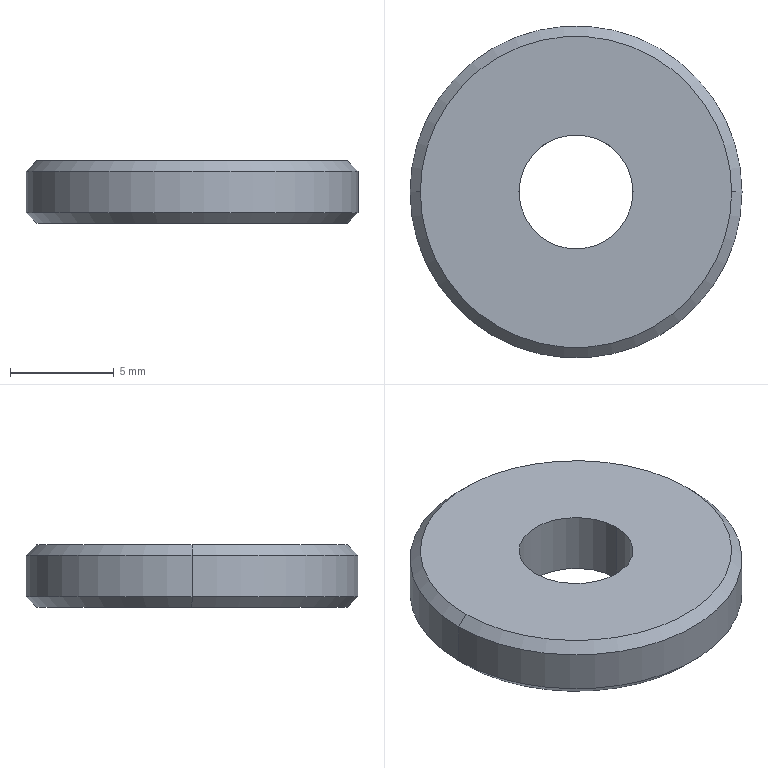Part | STEP file | 1 solid | 10 faces | box 16 x 16 x 3 mm | volume 519.606 mm3 | cone 4 | cylinder 4 | plane 2 | commonest cylinder face diameters 5.5 x2 16 x2
STEP:
#1=CARTESIAN_POINT('',(0.,0.,0.));
#2=DIRECTION('',(0.,0.,1.));
#3=DIRECTION('',(1.,0.,0.));
#4=AXIS2_PLACEMENT_3D('',#1,#2,#3);
#5=CARTESIAN_POINT('',(-7.5,0.,0.));
#6=VERTEX_POINT('',#5);
#7=CARTESIAN_POINT('',(7.5,0.,0.));
#8=VERTEX_POINT('',#7);
#9=CARTESIAN_POINT('',(0.,0.,0.));
#10=DIRECTION('',(0.,0.,-1.));
#11=DIRECTION('',(1.,0.,0.));
#12=AXIS2_PLACEMENT_3D('',#9,#10,#11);
#13=CIRCLE('',#12,7.5);
#14=CARTESIAN_POINT('',(0.,0.,0.5));
#15=DIRECTION('',(0.,0.,1.));
#16=DIRECTION('',(1.,0.,0.));
#17=AXIS2_PLACEMENT_3D('',#14,#15,#16);
#18=CONICAL_SURFACE('',#17,8.,0.7854);
#19=CARTESIAN_POINT('',(6.283,-0.5));
#20=DIRECTION('',(-1.,0.));
#21=VECTOR('',#20,1.);
#22=LINE('',#19,#21);
#23=(GEOMETRIC_REPRESENTATION_CONTEXT(2)PARAMETRIC_REPRESENTATION_CONTEXT()REPRESENTATION_CONTEXT('',''));
#24=DEFINITIONAL_REPRESENTATION('',(#22),#23);
#25=PCURVE('',#18,#24);
#26=CARTESIAN_POINT('',(0.,0.,0.));
#27=DIRECTION('',(0.,0.,1.));
#28=DIRECTION('',(1.,0.,0.));
#29=AXIS2_PLACEMENT_3D('',#26,#27,#28);
#30=PLANE('',#29);
#31=CARTESIAN_POINT('',(7.5,0.));
#32=CARTESIAN_POINT('',(7.5,-12.99));
#33=CARTESIAN_POINT('',(-3.75,-6.495));
#34=CARTESIAN_POINT('',(-15.,0.));
#35=CARTESIAN_POINT('',(-3.75,6.495));
#36=CARTESIAN_POINT('',(7.5,12.99));
#37=CARTESIAN_POINT('',(7.5,0.));
#38=(BOUNDED_CURVE()B_SPLINE_CURVE(2,(#31,#32,#33,#34,#35,#36,#37),.UNSPECIFIED.,.T.,.F.)B_SPLINE_CURVE_WITH_KNOTS((1,2,2,2,2,1),(-2.094,0.,2.094,4.189,6.283,8.378),.UNSPECIFIED.)CURVE()GEOMETRIC_REPRESENTATION_ITEM()RATIONAL_B_SPLINE_CURVE((1.,0.5,1.,0.5,1.,0.5,1.))REPRESENTATION_ITEM(''));
#39=(GEOMETRIC_REPRESENTATION_CONTEXT(2)PARAMETRIC_REPRESENTATION_CONTEXT()REPRESENTATION_CONTEXT('',''));
#40=DEFINITIONAL_REPRESENTATION('',(#38),#39);
#41=PCURVE('',#30,#40);
#42=SURFACE_CURVE('',#13,(#25,#41),.PCURVE_S1.);
#43=EDGE_CURVE('',#6,#8,#42,.T.);
#44=ORIENTED_EDGE('',*,*,#43,.F.);
#45=CARTESIAN_POINT('',(-8.,0.,0.5));
#46=VERTEX_POINT('',#45);
#47=CARTESIAN_POINT('',(-8.,0.,0.5));
#48=DIRECTION('',(-0.7071,0.,0.7071));
#49=VECTOR('',#48,1.);
#50=LINE('',#47,#49);
#51=CARTESIAN_POINT('',(3.142,0.));
#52=DIRECTION('',(0.,1.));
#53=VECTOR('',#52,1.);
#54=LINE('',#51,#53);
#55=(GEOMETRIC_REPRESENTATION_CONTEXT(2)PARAMETRIC_REPRESENTATION_CONTEXT()REPRESENTATION_CONTEXT('',''));
#56=DEFINITIONAL_REPRESENTATION('',(#54),#55);
#57=PCURVE('',#18,#56);
#58=CARTESIAN_POINT('',(0.,0.,0.5));
#59=DIRECTION('',(0.,0.,1.));
#60=DIRECTION('',(1.,0.,0.));
#61=AXIS2_PLACEMENT_3D('',#58,#59,#60);
#62=CONICAL_SURFACE('',#61,8.,0.7854);
#63=CARTESIAN_POINT('',(3.142,0.));
#64=DIRECTION('',(0.,1.));
#65=VECTOR('',#64,1.);
#66=LINE('',#63,#65);
#67=(GEOMETRIC_REPRESENTATION_CONTEXT(2)PARAMETRIC_REPRESENTATION_CONTEXT()REPRESENTATION_CONTEXT('',''));
#68=DEFINITIONAL_REPRESENTATION('',(#66),#67);
#69=PCURVE('',#62,#68);
#70=SURFACE_CURVE('',#50,(#57,#69),.PCURVE_S1.);
#71=EDGE_CURVE('',#6,#46,#70,.T.);
#72=ORIENTED_EDGE('',*,*,#71,.T.);
#73=CARTESIAN_POINT('',(8.,0.,0.5));
#74=VERTEX_POINT('',#73);
#75=CARTESIAN_POINT('',(0.,0.,0.5));
#76=DIRECTION('',(0.,0.,1.));
#77=DIRECTION('',(1.,0.,0.));
#78=AXIS2_PLACEMENT_3D('',#75,#76,#77);
#79=CIRCLE('',#78,8.);
#80=CARTESIAN_POINT('',(0.,0.));
#81=DIRECTION('',(1.,0.));
#82=VECTOR('',#81,1.);
#83=LINE('',#80,#82);
#84=(GEOMETRIC_REPRESENTATION_CONTEXT(2)PARAMETRIC_REPRESENTATION_CONTEXT()REPRESENTATION_CONTEXT('',''));
#85=DEFINITIONAL_REPRESENTATION('',(#83),#84);
#86=PCURVE('',#18,#85);
#87=CARTESIAN_POINT('',(0.,0.,3.));
#88=DIRECTION('',(0.,0.,-1.));
#89=DIRECTION('',(-1.,0.,0.));
#90=AXIS2_PLACEMENT_3D('',#87,#88,#89);
#91=CYLINDRICAL_SURFACE('',#90,8.);
#92=CARTESIAN_POINT('',(3.142,2.5));
#93=DIRECTION('',(-1.,0.));
#94=VECTOR('',#93,1.);
#95=LINE('',#92,#94);
#96=(GEOMETRIC_REPRESENTATION_CONTEXT(2)PARAMETRIC_REPRESENTATION_CONTEXT()REPRESENTATION_CONTEXT('',''));
#97=DEFINITIONAL_REPRESENTATION('',(#95),#96);
#98=PCURVE('',#91,#97);
#99=SURFACE_CURVE('',#79,(#86,#98),.PCURVE_S1.);
#100=EDGE_CURVE('',#74,#46,#99,.T.);
#101=ORIENTED_EDGE('',*,*,#100,.F.);
#102=CARTESIAN_POINT('',(8.,0.,0.5));
#103=DIRECTION('',(0.7071,0.,0.7071));
#104=VECTOR('',#103,1.);
#105=LINE('',#102,#104);
#106=CARTESIAN_POINT('',(0.,0.));
#107=DIRECTION('',(0.,1.));
#108=VECTOR('',#107,1.);
#109=LINE('',#106,#108);
#110=(GEOMETRIC_REPRESENTATION_CONTEXT(2)PARAMETRIC_REPRESENTATION_CONTEXT()REPRESENTATION_CONTEXT('',''));
#111=DEFINITIONAL_REPRESENTATION('',(#109),#110);
#112=PCURVE('',#18,#111);
#113=CARTESIAN_POINT('',(6.283,0.));
#114=DIRECTION('',(0.,1.));
#115=VECTOR('',#114,1.);
#116=LINE('',#113,#115);
#117=(GEOMETRIC_REPRESENTATION_CONTEXT(2)PARAMETRIC_REPRESENTATION_CONTEXT()REPRESENTATION_CONTEXT('',''));
#118=DEFINITIONAL_REPRESENTATION('',(#116),#117);
#119=PCURVE('',#62,#118);
#120=SURFACE_CURVE('',#105,(#112,#119),.PCURVE_S1.);
#121=EDGE_CURVE('',#8,#74,#120,.T.);
#122=ORIENTED_EDGE('',*,*,#121,.F.);
#123=EDGE_LOOP('',(#44,#72,#101,#122));
#124=FACE_BOUND('',#123,.T.);
#125=ADVANCED_FACE('',(#124),#18,.T.);
#126=CARTESIAN_POINT('',(7.5,0.,3.));
#127=VERTEX_POINT('',#126);
#128=CARTESIAN_POINT('',(-7.5,0.,3.));
#129=VERTEX_POINT('',#128);
#130=CARTESIAN_POINT('',(0.,0.,3.));
#131=DIRECTION('',(0.,0.,1.));
#132=DIRECTION('',(1.,0.,0.));
#133=AXIS2_PLACEMENT_3D('',#130,#131,#132);
#134=CIRCLE('',#133,7.5);
#135=CARTESIAN_POINT('',(0.,0.,3.));
#136=DIRECTION('',(0.,0.,-1.));
#137=DIRECTION('',(-1.,0.,0.));
#138=AXIS2_PLACEMENT_3D('',#135,#136,#137);
#139=CONICAL_SURFACE('',#138,7.5,0.7854);
#140=CARTESIAN_POINT('',(3.142,0.));
#141=DIRECTION('',(-1.,0.));
#142=VECTOR('',#141,1.);
#143=LINE('',#140,#142);
#144=(GEOMETRIC_REPRESENTATION_CONTEXT(2)PARAMETRIC_REPRESENTATION_CONTEXT()REPRESENTATION_CONTEXT('',''));
#145=DEFINITIONAL_REPRESENTATION('',(#143),#144);
#146=PCURVE('',#139,#145);
#147=CARTESIAN_POINT('',(0.,0.,3.));
#148=DIRECTION('',(0.,0.,1.));
#149=DIRECTION('',(1.,0.,0.));
#150=AXIS2_PLACEMENT_3D('',#147,#148,#149);
#151=PLANE('',#150);
#152=CARTESIAN_POINT('',(0.,0.));
#153=DIRECTION('',(1.,0.));
#154=AXIS2_PLACEMENT_2D('',#152,#153);
#155=CIRCLE('',#154,7.5);
#156=(GEOMETRIC_REPRESENTATION_CONTEXT(2)PARAMETRIC_REPRESENTATION_CONTEXT()REPRESENTATION_CONTEXT('',''));
#157=DEFINITIONAL_REPRESENTATION('',(#155),#156);
#158=PCURVE('',#151,#157);
#159=SURFACE_CURVE('',#134,(#146,#158),.PCURVE_S1.);
#160=EDGE_CURVE('',#127,#129,#159,.T.);
#161=ORIENTED_EDGE('',*,*,#160,.F.);
#162=CARTESIAN_POINT('',(8.,0.,2.5));
#163=VERTEX_POINT('',#162);
#164=CARTESIAN_POINT('',(7.5,0.,3.));
#165=DIRECTION('',(0.7071,0.,-0.7071));
#166=VECTOR('',#165,1.);
#167=LINE('',#164,#166);
#168=CARTESIAN_POINT('',(3.142,0.));
#169=DIRECTION('',(0.,1.));
#170=VECTOR('',#169,1.);
#171=LINE('',#168,#170);
#172=(GEOMETRIC_REPRESENTATION_CONTEXT(2)PARAMETRIC_REPRESENTATION_CONTEXT()REPRESENTATION_CONTEXT('',''));
#173=DEFINITIONAL_REPRESENTATION('',(#171),#172);
#174=PCURVE('',#139,#173);
#175=CARTESIAN_POINT('',(0.,0.,3.));
#176=DIRECTION('',(0.,0.,-1.));
#177=DIRECTION('',(-1.,0.,0.));
#178=AXIS2_PLACEMENT_3D('',#175,#176,#177);
#179=CONICAL_SURFACE('',#178,7.5,0.7854);
#180=CARTESIAN_POINT('',(3.142,0.));
#181=DIRECTION('',(0.,1.));
#182=VECTOR('',#181,1.);
#183=LINE('',#180,#182);
#184=(GEOMETRIC_REPRESENTATION_CONTEXT(2)PARAMETRIC_REPRESENTATION_CONTEXT()REPRESENTATION_CONTEXT('',''));
#185=DEFINITIONAL_REPRESENTATION('',(#183),#184);
#186=PCURVE('',#179,#185);
#187=SURFACE_CURVE('',#167,(#174,#186),.PCURVE_S1.);
#188=EDGE_CURVE('',#127,#163,#187,.T.);
#189=ORIENTED_EDGE('',*,*,#188,.T.);
#190=CARTESIAN_POINT('',(-8.,0.,2.5));
#191=VERTEX_POINT('',#190);
#192=CARTESIAN_POINT('',(0.,0.,2.5));
#193=DIRECTION('',(0.,0.,-1.));
#194=DIRECTION('',(1.,0.,0.));
#195=AXIS2_PLACEMENT_3D('',#192,#193,#194);
#196=CIRCLE('',#195,8.);
#197=CARTESIAN_POINT('',(-3.142,0.5));
#198=DIRECTION('',(1.,0.));
#199=VECTOR('',#198,1.);
#200=LINE('',#197,#199);
#201=(GEOMETRIC_REPRESENTATION_CONTEXT(2)PARAMETRIC_REPRESENTATION_CONTEXT()REPRESENTATION_CONTEXT('',''));
#202=DEFINITIONAL_REPRESENTATION('',(#200),#201);
#203=PCURVE('',#139,#202);
#204=CARTESIAN_POINT('',(-3.142,0.5));
#205=DIRECTION('',(1.,0.));
#206=VECTOR('',#205,1.);
#207=LINE('',#204,#206);
#208=(GEOMETRIC_REPRESENTATION_CONTEXT(2)PARAMETRIC_REPRESENTATION_CONTEXT()REPRESENTATION_CONTEXT('',''));
#209=DEFINITIONAL_REPRESENTATION('',(#207),#208);
#210=PCURVE('',#91,#209);
#211=SURFACE_CURVE('',#196,(#203,#210),.PCURVE_S1.);
#212=EDGE_CURVE('',#191,#163,#211,.T.);
#213=ORIENTED_EDGE('',*,*,#212,.F.);
#214=CARTESIAN_POINT('',(-7.5,0.,3.));
#215=DIRECTION('',(-0.7071,0.,-0.7071));
#216=VECTOR('',#215,1.);
#217=LINE('',#214,#216);
#218=CARTESIAN_POINT('',(0.,0.));
#219=DIRECTION('',(0.,1.));
#220=VECTOR('',#219,1.);
#221=LINE('',#218,#220);
#222=(GEOMETRIC_REPRESENTATION_CONTEXT(2)PARAMETRIC_REPRESENTATION_CONTEXT()REPRESENTATION_CONTEXT('',''));
#223=DEFINITIONAL_REPRESENTATION('',(#221),#222);
#224=PCURVE('',#139,#223);
#225=CARTESIAN_POINT('',(6.283,0.));
#226=DIRECTION('',(0.,1.));
#227=VECTOR('',#226,1.);
#228=LINE('',#225,#227);
#229=(GEOMETRIC_REPRESENTATION_CONTEXT(2)PARAMETRIC_REPRESENTATION_CONTEXT()REPRESENTATION_CONTEXT('',''));
#230=DEFINITIONAL_REPRESENTATION('',(#228),#229);
#231=PCURVE('',#179,#230);
#232=SURFACE_CURVE('',#217,(#224,#231),.PCURVE_S1.);
#233=EDGE_CURVE('',#129,#191,#232,.T.);
#234=ORIENTED_EDGE('',*,*,#233,.F.);
#235=EDGE_LOOP('',(#161,#189,#213,#234));
#236=FACE_BOUND('',#235,.T.);
#237=ADVANCED_FACE('',(#236),#139,.T.);
#238=CARTESIAN_POINT('',(-2.75,0.,3.));
#239=VERTEX_POINT('',#238);
#240=CARTESIAN_POINT('',(-2.75,0.,0.));
#241=VERTEX_POINT('',#240);
#242=CARTESIAN_POINT('',(-2.75,0.,3.));
#243=DIRECTION('',(0.,0.,-1.));
#244=VECTOR('',#243,1.);
#245=LINE('',#242,#244);
#246=CARTESIAN_POINT('',(0.,0.,3.));
#247=DIRECTION('',(0.,0.,-1.));
#248=DIRECTION('',(-1.,0.,0.));
#249=AXIS2_PLACEMENT_3D('',#246,#247,#248);
#250=CYLINDRICAL_SURFACE('',#249,2.75);
#251=CARTESIAN_POINT('',(6.283,0.));
#252=DIRECTION('',(0.,1.));
#253=VECTOR('',#252,1.);
#254=LINE('',#251,#253);
#255=(GEOMETRIC_REPRESENTATION_CONTEXT(2)PARAMETRIC_REPRESENTATION_CONTEXT()REPRESENTATION_CONTEXT('',''));
#256=DEFINITIONAL_REPRESENTATION('',(#254),#255);
#257=PCURVE('',#250,#256);
#258=CARTESIAN_POINT('',(0.,0.,3.));
#259=DIRECTION('',(0.,0.,-1.));
#260=DIRECTION('',(-1.,0.,0.));
#261=AXIS2_PLACEMENT_3D('',#258,#259,#260);
#262=CYLINDRICAL_SURFACE('',#261,2.75);
#263=CARTESIAN_POINT('',(0.,0.));
#264=DIRECTION('',(0.,1.));
#265=VECTOR('',#264,1.);
#266=LINE('',#263,#265);
#267=(GEOMETRIC_REPRESENTATION_CONTEXT(2)PARAMETRIC_REPRESENTATION_CONTEXT()REPRESENTATION_CONTEXT('',''));
#268=DEFINITIONAL_REPRESENTATION('',(#266),#267);
#269=PCURVE('',#262,#268);
#270=SURFACE_CURVE('',#245,(#257,#269),.PCURVE_S1.);
#271=EDGE_CURVE('',#239,#241,#270,.T.);
#272=ORIENTED_EDGE('',*,*,#271,.T.);
#273=CARTESIAN_POINT('',(2.75,0.,0.));
#274=VERTEX_POINT('',#273);
#275=CARTESIAN_POINT('',(0.,0.,0.));
#276=DIRECTION('',(0.,0.,1.));
#277=DIRECTION('',(1.,0.,0.));
#278=AXIS2_PLACEMENT_3D('',#275,#276,#277);
#279=CIRCLE('',#278,2.75);
#280=CARTESIAN_POINT('',(9.425,3.));
#281=DIRECTION('',(-1.,0.));
#282=VECTOR('',#281,1.);
#283=LINE('',#280,#282);
#284=(GEOMETRIC_REPRESENTATION_CONTEXT(2)PARAMETRIC_REPRESENTATION_CONTEXT()REPRESENTATION_CONTEXT('',''));
#285=DEFINITIONAL_REPRESENTATION('',(#283),#284);
#286=PCURVE('',#250,#285);
#287=CARTESIAN_POINT('',(0.,0.));
#288=DIRECTION('',(1.,0.));
#289=AXIS2_PLACEMENT_2D('',#287,#288);
#290=CIRCLE('',#289,2.75);
#291=(GEOMETRIC_REPRESENTATION_CONTEXT(2)PARAMETRIC_REPRESENTATION_CONTEXT()REPRESENTATION_CONTEXT('',''));
#292=DEFINITIONAL_REPRESENTATION('',(#290),#291);
#293=PCURVE('',#30,#292);
#294=SURFACE_CURVE('',#279,(#286,#293),.PCURVE_S1.);
#295=EDGE_CURVE('',#241,#274,#294,.T.);
#296=ORIENTED_EDGE('',*,*,#295,.T.);
#297=CARTESIAN_POINT('',(2.75,0.,3.));
#298=VERTEX_POINT('',#297);
#299=CARTESIAN_POINT('',(2.75,0.,3.));
#300=DIRECTION('',(0.,0.,-1.));
#301=VECTOR('',#300,1.);
#302=LINE('',#299,#301);
#303=CARTESIAN_POINT('',(3.142,0.));
#304=DIRECTION('',(0.,1.));
#305=VECTOR('',#304,1.);
#306=LINE('',#303,#305);
#307=(GEOMETRIC_REPRESENTATION_CONTEXT(2)PARAMETRIC_REPRESENTATION_CONTEXT()REPRESENTATION_CONTEXT('',''));
#308=DEFINITIONAL_REPRESENTATION('',(#306),#307);
#309=PCURVE('',#250,#308);
#310=CARTESIAN_POINT('',(3.142,0.));
#311=DIRECTION('',(0.,1.));
#312=VECTOR('',#311,1.);
#313=LINE('',#310,#312);
#314=(GEOMETRIC_REPRESENTATION_CONTEXT(2)PARAMETRIC_REPRESENTATION_CONTEXT()REPRESENTATION_CONTEXT('',''));
#315=DEFINITIONAL_REPRESENTATION('',(#313),#314);
#316=PCURVE('',#262,#315);
#317=SURFACE_CURVE('',#302,(#309,#316),.PCURVE_S1.);
#318=EDGE_CURVE('',#298,#274,#317,.T.);
#319=ORIENTED_EDGE('',*,*,#318,.F.);
#320=CARTESIAN_POINT('',(0.,0.,3.));
#321=DIRECTION('',(0.,0.,1.));
#322=DIRECTION('',(1.,0.,0.));
#323=AXIS2_PLACEMENT_3D('',#320,#321,#322);
#324=CIRCLE('',#323,2.75);
#325=CARTESIAN_POINT('',(9.425,0.));
#326=DIRECTION('',(-1.,0.));
#327=VECTOR('',#326,1.);
#328=LINE('',#325,#327);
#329=(GEOMETRIC_REPRESENTATION_CONTEXT(2)PARAMETRIC_REPRESENTATION_CONTEXT()REPRESENTATION_CONTEXT('',''));
#330=DEFINITIONAL_REPRESENTATION('',(#328),#329);
#331=PCURVE('',#250,#330);
#332=CARTESIAN_POINT('',(0.,0.));
#333=DIRECTION('',(1.,0.));
#334=AXIS2_PLACEMENT_2D('',#332,#333);
#335=CIRCLE('',#334,2.75);
#336=(GEOMETRIC_REPRESENTATION_CONTEXT(2)PARAMETRIC_REPRESENTATION_CONTEXT()REPRESENTATION_CONTEXT('',''));
#337=DEFINITIONAL_REPRESENTATION('',(#335),#336);
#338=PCURVE('',#151,#337);
#339=SURFACE_CURVE('',#324,(#331,#338),.PCURVE_S1.);
#340=EDGE_CURVE('',#239,#298,#339,.T.);
#341=ORIENTED_EDGE('',*,*,#340,.F.);
#342=EDGE_LOOP('',(#272,#296,#319,#341));
#343=FACE_BOUND('',#342,.F.);
#344=ADVANCED_FACE('',(#343),#250,.F.);
#345=ORIENTED_EDGE('',*,*,#212,.T.);
#346=CARTESIAN_POINT('',(8.,0.,3.));
#347=DIRECTION('',(0.,0.,-1.));
#348=VECTOR('',#347,1.);
#349=LINE('',#346,#348);
#350=CARTESIAN_POINT('',(3.142,0.));
#351=DIRECTION('',(0.,1.));
#352=VECTOR('',#351,1.);
#353=LINE('',#350,#352);
#354=(GEOMETRIC_REPRESENTATION_CONTEXT(2)PARAMETRIC_REPRESENTATION_CONTEXT()REPRESENTATION_CONTEXT('',''));
#355=DEFINITIONAL_REPRESENTATION('',(#353),#354);
#356=PCURVE('',#91,#355);
#357=CARTESIAN_POINT('',(0.,0.,3.));
#358=DIRECTION('',(0.,0.,-1.));
#359=DIRECTION('',(-1.,0.,0.));
#360=AXIS2_PLACEMENT_3D('',#357,#358,#359);
#361=CYLINDRICAL_SURFACE('',#360,8.);
#362=CARTESIAN_POINT('',(3.142,0.));
#363=DIRECTION('',(0.,1.));
#364=VECTOR('',#363,1.);
#365=LINE('',#362,#364);
#366=(GEOMETRIC_REPRESENTATION_CONTEXT(2)PARAMETRIC_REPRESENTATION_CONTEXT()REPRESENTATION_CONTEXT('',''));
#367=DEFINITIONAL_REPRESENTATION('',(#365),#366);
#368=PCURVE('',#361,#367);
#369=SURFACE_CURVE('',#349,(#356,#368),.PCURVE_S1.);
#370=EDGE_CURVE('',#163,#74,#369,.T.);
#371=ORIENTED_EDGE('',*,*,#370,.T.);
#372=ORIENTED_EDGE('',*,*,#100,.T.);
#373=CARTESIAN_POINT('',(-8.,0.,3.));
#374=DIRECTION('',(0.,0.,-1.));
#375=VECTOR('',#374,1.);
#376=LINE('',#373,#375);
#377=CARTESIAN_POINT('',(0.,0.));
#378=DIRECTION('',(0.,1.));
#379=VECTOR('',#378,1.);
#380=LINE('',#377,#379);
#381=(GEOMETRIC_REPRESENTATION_CONTEXT(2)PARAMETRIC_REPRESENTATION_CONTEXT()REPRESENTATION_CONTEXT('',''));
#382=DEFINITIONAL_REPRESENTATION('',(#380),#381);
#383=PCURVE('',#91,#382);
#384=CARTESIAN_POINT('',(6.283,0.));
#385=DIRECTION('',(0.,1.));
#386=VECTOR('',#385,1.);
#387=LINE('',#384,#386);
#388=(GEOMETRIC_REPRESENTATION_CONTEXT(2)PARAMETRIC_REPRESENTATION_CONTEXT()REPRESENTATION_CONTEXT('',''));
#389=DEFINITIONAL_REPRESENTATION('',(#387),#388);
#390=PCURVE('',#361,#389);
#391=SURFACE_CURVE('',#376,(#383,#390),.PCURVE_S1.);
#392=EDGE_CURVE('',#191,#46,#391,.T.);
#393=ORIENTED_EDGE('',*,*,#392,.F.);
#394=EDGE_LOOP('',(#345,#371,#372,#393));
#395=FACE_BOUND('',#394,.T.);
#396=ADVANCED_FACE('',(#395),#91,.T.);
#397=CARTESIAN_POINT('',(0.,0.,3.));
#398=DIRECTION('',(0.,0.,1.));
#399=DIRECTION('',(1.,0.,0.));
#400=AXIS2_PLACEMENT_3D('',#397,#398,#399);
#401=CIRCLE('',#400,7.5);
#402=CARTESIAN_POINT('',(0.,0.));
#403=DIRECTION('',(1.,0.));
#404=AXIS2_PLACEMENT_2D('',#402,#403);
#405=CIRCLE('',#404,7.5);
#406=(GEOMETRIC_REPRESENTATION_CONTEXT(2)PARAMETRIC_REPRESENTATION_CONTEXT()REPRESENTATION_CONTEXT('',''));
#407=DEFINITIONAL_REPRESENTATION('',(#405),#406);
#408=PCURVE('',#151,#407);
#409=CARTESIAN_POINT('',(9.425,0.));
#410=DIRECTION('',(-1.,0.));
#411=VECTOR('',#410,1.);
#412=LINE('',#409,#411);
#413=(GEOMETRIC_REPRESENTATION_CONTEXT(2)PARAMETRIC_REPRESENTATION_CONTEXT()REPRESENTATION_CONTEXT('',''));
#414=DEFINITIONAL_REPRESENTATION('',(#412),#413);
#415=PCURVE('',#179,#414);
#416=SURFACE_CURVE('',#401,(#408,#415),.PCURVE_S1.);
#417=EDGE_CURVE('',#129,#127,#416,.T.);
#418=ORIENTED_EDGE('',*,*,#417,.T.);
#419=ORIENTED_EDGE('',*,*,#160,.T.);
#420=EDGE_LOOP('',(#418,#419));
#421=FACE_BOUND('',#420,.T.);
#422=ORIENTED_EDGE('',*,*,#340,.F.);
#423=CARTESIAN_POINT('',(0.,0.,3.));
#424=DIRECTION('',(0.,0.,1.));
#425=DIRECTION('',(1.,0.,0.));
#426=AXIS2_PLACEMENT_3D('',#423,#424,#425);
#427=CIRCLE('',#426,2.75);
#428=CARTESIAN_POINT('',(0.,0.));
#429=DIRECTION('',(1.,0.));
#430=AXIS2_PLACEMENT_2D('',#428,#429);
#431=CIRCLE('',#430,2.75);
#432=(GEOMETRIC_REPRESENTATION_CONTEXT(2)PARAMETRIC_REPRESENTATION_CONTEXT()REPRESENTATION_CONTEXT('',''));
#433=DEFINITIONAL_REPRESENTATION('',(#431),#432);
#434=PCURVE('',#151,#433);
#435=CARTESIAN_POINT('',(3.142,0.));
#436=DIRECTION('',(-1.,0.));
#437=VECTOR('',#436,1.);
#438=LINE('',#435,#437);
#439=(GEOMETRIC_REPRESENTATION_CONTEXT(2)PARAMETRIC_REPRESENTATION_CONTEXT()REPRESENTATION_CONTEXT('',''));
#440=DEFINITIONAL_REPRESENTATION('',(#438),#439);
#441=PCURVE('',#262,#440);
#442=SURFACE_CURVE('',#427,(#434,#441),.PCURVE_S1.);
#443=EDGE_CURVE('',#298,#239,#442,.T.);
#444=ORIENTED_EDGE('',*,*,#443,.F.);
#445=EDGE_LOOP('',(#422,#444));
#446=FACE_BOUND('',#445,.T.);
#447=ADVANCED_FACE('',(#421,#446),#151,.T.);
#448=CARTESIAN_POINT('',(0.,0.,0.));
#449=DIRECTION('',(0.,0.,-1.));
#450=DIRECTION('',(1.,0.,0.));
#451=AXIS2_PLACEMENT_3D('',#448,#449,#450);
#452=CIRCLE('',#451,7.5);
#453=CARTESIAN_POINT('',(7.5,0.));
#454=CARTESIAN_POINT('',(7.5,-12.99));
#455=CARTESIAN_POINT('',(-3.75,-6.495));
#456=CARTESIAN_POINT('',(-15.,0.));
#457=CARTESIAN_POINT('',(-3.75,6.495));
#458=CARTESIAN_POINT('',(7.5,12.99));
#459=CARTESIAN_POINT('',(7.5,0.));
#460=(BOUNDED_CURVE()B_SPLINE_CURVE(2,(#453,#454,#455,#456,#457,#458,#459),.UNSPECIFIED.,.T.,.F.)B_SPLINE_CURVE_WITH_KNOTS((1,2,2,2,2,1),(-2.094,0.,2.094,4.189,6.283,8.378),.UNSPECIFIED.)CURVE()GEOMETRIC_REPRESENTATION_ITEM()RATIONAL_B_SPLINE_CURVE((1.,0.5,1.,0.5,1.,0.5,1.))REPRESENTATION_ITEM(''));
#461=(GEOMETRIC_REPRESENTATION_CONTEXT(2)PARAMETRIC_REPRESENTATION_CONTEXT()REPRESENTATION_CONTEXT('',''));
#462=DEFINITIONAL_REPRESENTATION('',(#460),#461);
#463=PCURVE('',#30,#462);
#464=CARTESIAN_POINT('',(6.283,-0.5));
#465=DIRECTION('',(-1.,0.));
#466=VECTOR('',#465,1.);
#467=LINE('',#464,#466);
#468=(GEOMETRIC_REPRESENTATION_CONTEXT(2)PARAMETRIC_REPRESENTATION_CONTEXT()REPRESENTATION_CONTEXT('',''));
#469=DEFINITIONAL_REPRESENTATION('',(#467),#468);
#470=PCURVE('',#62,#469);
#471=SURFACE_CURVE('',#452,(#463,#470),.PCURVE_S1.);
#472=EDGE_CURVE('',#8,#6,#471,.T.);
#473=ORIENTED_EDGE('',*,*,#472,.T.);
#474=ORIENTED_EDGE('',*,*,#43,.T.);
#475=EDGE_LOOP('',(#473,#474));
#476=FACE_BOUND('',#475,.T.);
#477=ORIENTED_EDGE('',*,*,#295,.T.);
#478=CARTESIAN_POINT('',(0.,0.,0.));
#479=DIRECTION('',(0.,0.,1.));
#480=DIRECTION('',(1.,0.,0.));
#481=AXIS2_PLACEMENT_3D('',#478,#479,#480);
#482=CIRCLE('',#481,2.75);
#483=CARTESIAN_POINT('',(0.,0.));
#484=DIRECTION('',(1.,0.));
#485=AXIS2_PLACEMENT_2D('',#483,#484);
#486=CIRCLE('',#485,2.75);
#487=(GEOMETRIC_REPRESENTATION_CONTEXT(2)PARAMETRIC_REPRESENTATION_CONTEXT()REPRESENTATION_CONTEXT('',''));
#488=DEFINITIONAL_REPRESENTATION('',(#486),#487);
#489=PCURVE('',#30,#488);
#490=CARTESIAN_POINT('',(3.142,3.));
#491=DIRECTION('',(-1.,0.));
#492=VECTOR('',#491,1.);
#493=LINE('',#490,#492);
#494=(GEOMETRIC_REPRESENTATION_CONTEXT(2)PARAMETRIC_REPRESENTATION_CONTEXT()REPRESENTATION_CONTEXT('',''));
#495=DEFINITIONAL_REPRESENTATION('',(#493),#494);
#496=PCURVE('',#262,#495);
#497=SURFACE_CURVE('',#482,(#489,#496),.PCURVE_S1.);
#498=EDGE_CURVE('',#274,#241,#497,.T.);
#499=ORIENTED_EDGE('',*,*,#498,.T.);
#500=EDGE_LOOP('',(#477,#499));
#501=FACE_BOUND('',#500,.T.);
#502=ADVANCED_FACE('',(#476,#501),#30,.F.);
#503=ORIENTED_EDGE('',*,*,#370,.F.);
#504=CARTESIAN_POINT('',(0.,0.,2.5));
#505=DIRECTION('',(0.,0.,-1.));
#506=DIRECTION('',(1.,0.,0.));
#507=AXIS2_PLACEMENT_3D('',#504,#505,#506);
#508=CIRCLE('',#507,8.);
#509=CARTESIAN_POINT('',(3.142,0.5));
#510=DIRECTION('',(1.,0.));
#511=VECTOR('',#510,1.);
#512=LINE('',#509,#511);
#513=(GEOMETRIC_REPRESENTATION_CONTEXT(2)PARAMETRIC_REPRESENTATION_CONTEXT()REPRESENTATION_CONTEXT('',''));
#514=DEFINITIONAL_REPRESENTATION('',(#512),#513);
#515=PCURVE('',#361,#514);
#516=CARTESIAN_POINT('',(3.142,0.5));
#517=DIRECTION('',(1.,0.));
#518=VECTOR('',#517,1.);
#519=LINE('',#516,#518);
#520=(GEOMETRIC_REPRESENTATION_CONTEXT(2)PARAMETRIC_REPRESENTATION_CONTEXT()REPRESENTATION_CONTEXT('',''));
#521=DEFINITIONAL_REPRESENTATION('',(#519),#520);
#522=PCURVE('',#179,#521);
#523=SURFACE_CURVE('',#508,(#515,#522),.PCURVE_S1.);
#524=EDGE_CURVE('',#163,#191,#523,.T.);
#525=ORIENTED_EDGE('',*,*,#524,.T.);
#526=ORIENTED_EDGE('',*,*,#392,.T.);
#527=CARTESIAN_POINT('',(0.,0.,0.5));
#528=DIRECTION('',(0.,0.,1.));
#529=DIRECTION('',(1.,0.,0.));
#530=AXIS2_PLACEMENT_3D('',#527,#528,#529);
#531=CIRCLE('',#530,8.);
#532=CARTESIAN_POINT('',(9.425,2.5));
#533=DIRECTION('',(-1.,0.));
#534=VECTOR('',#533,1.);
#535=LINE('',#532,#534);
#536=(GEOMETRIC_REPRESENTATION_CONTEXT(2)PARAMETRIC_REPRESENTATION_CONTEXT()REPRESENTATION_CONTEXT('',''));
#537=DEFINITIONAL_REPRESENTATION('',(#535),#536);
#538=PCURVE('',#361,#537);
#539=CARTESIAN_POINT('',(0.,0.));
#540=DIRECTION('',(1.,0.));
#541=VECTOR('',#540,1.);
#542=LINE('',#539,#541);
#543=(GEOMETRIC_REPRESENTATION_CONTEXT(2)PARAMETRIC_REPRESENTATION_CONTEXT()REPRESENTATION_CONTEXT('',''));
#544=DEFINITIONAL_REPRESENTATION('',(#542),#543);
#545=PCURVE('',#62,#544);
#546=SURFACE_CURVE('',#531,(#538,#545),.PCURVE_S1.);
#547=EDGE_CURVE('',#46,#74,#546,.T.);
#548=ORIENTED_EDGE('',*,*,#547,.T.);
#549=EDGE_LOOP('',(#503,#525,#526,#548));
#550=FACE_BOUND('',#549,.T.);
#551=ADVANCED_FACE('',(#550),#361,.T.);
#552=ORIENTED_EDGE('',*,*,#498,.T.);
#553=ORIENTED_EDGE('',*,*,#271,.F.);
#554=ORIENTED_EDGE('',*,*,#443,.F.);
#555=ORIENTED_EDGE('',*,*,#318,.T.);
#556=EDGE_LOOP('',(#552,#553,#554,#555));
#557=FACE_BOUND('',#556,.F.);
#558=ADVANCED_FACE('',(#557),#262,.F.);
#559=ORIENTED_EDGE('',*,*,#188,.F.);
#560=ORIENTED_EDGE('',*,*,#417,.F.);
#561=ORIENTED_EDGE('',*,*,#233,.T.);
#562=ORIENTED_EDGE('',*,*,#524,.F.);
#563=EDGE_LOOP('',(#559,#560,#561,#562));
#564=FACE_BOUND('',#563,.T.);
#565=ADVANCED_FACE('',(#564),#179,.T.);
#566=ORIENTED_EDGE('',*,*,#71,.F.);
#567=ORIENTED_EDGE('',*,*,#472,.F.);
#568=ORIENTED_EDGE('',*,*,#121,.T.);
#569=ORIENTED_EDGE('',*,*,#547,.F.);
#570=EDGE_LOOP('',(#566,#567,#568,#569));
#571=FACE_BOUND('',#570,.T.);
#572=ADVANCED_FACE('',(#571),#62,.T.);
#573=CLOSED_SHELL('',(#125,#237,#344,#396,#447,#502,#551,#558,#565,#572));
#574=MANIFOLD_SOLID_BREP('',#573);
#575=(LENGTH_UNIT()NAMED_UNIT(*)SI_UNIT(.MILLI.,.METRE.));
#576=UNCERTAINTY_MEASURE_WITH_UNIT(LENGTH_MEASURE(0.0000001),#575,'','');
#577=(NAMED_UNIT(*)PLANE_ANGLE_UNIT()SI_UNIT($,.RADIAN.));
#578=(NAMED_UNIT(*)SI_UNIT($,.STERADIAN.)SOLID_ANGLE_UNIT());
#579=(GEOMETRIC_REPRESENTATION_CONTEXT(3)GLOBAL_UNCERTAINTY_ASSIGNED_CONTEXT((#576))GLOBAL_UNIT_ASSIGNED_CONTEXT((#575,#577,#578))REPRESENTATION_CONTEXT('',''));
#580=ADVANCED_BREP_SHAPE_REPRESENTATION('',(#4,#574),#579);